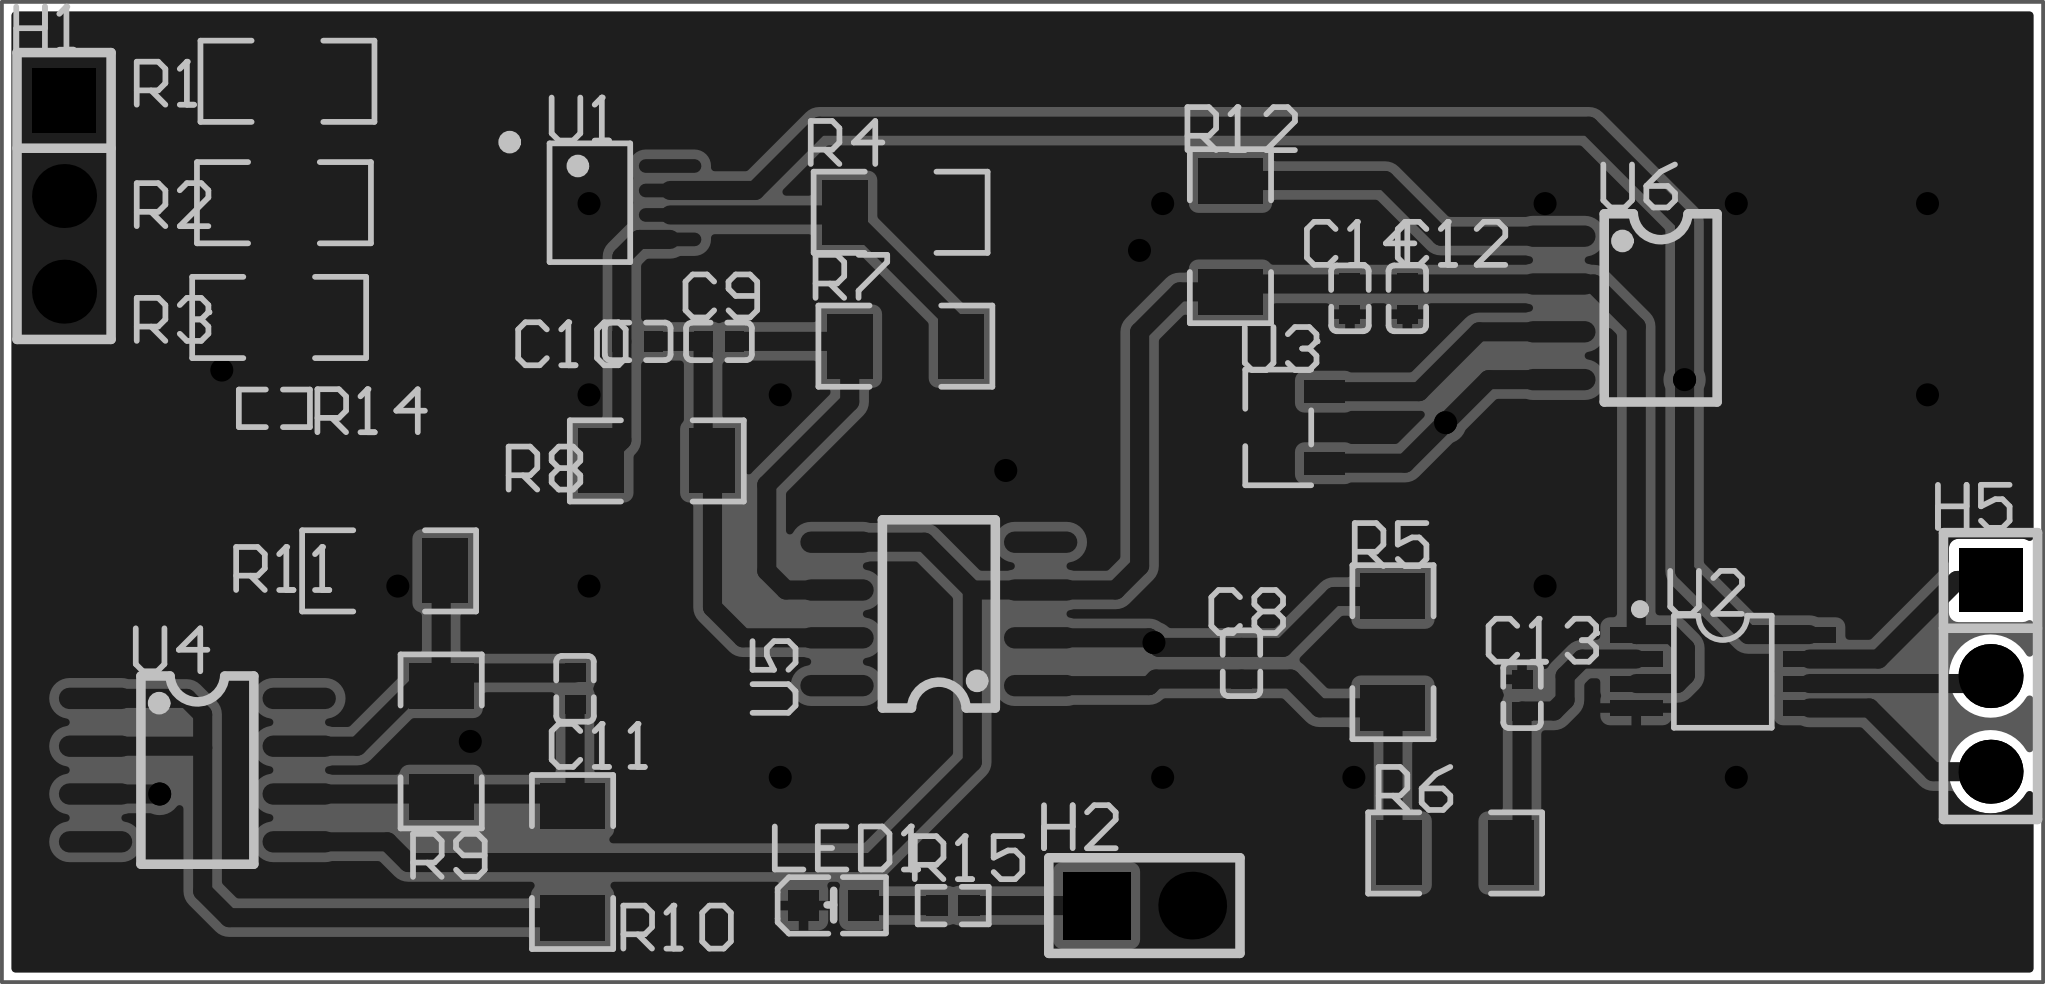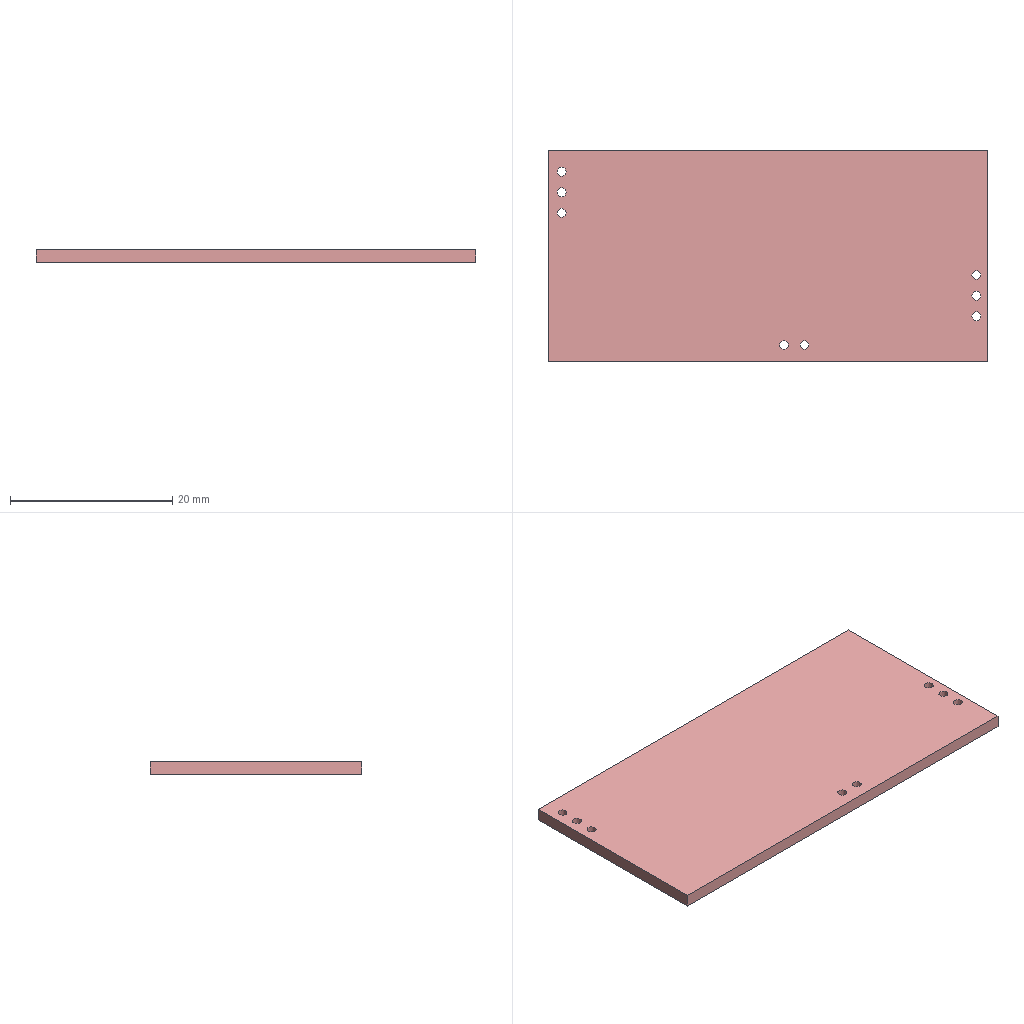Circuit board layout | Altium Designer | box 54.2 x 26 x 1.6 mm
Layer stack:
# Altium Designer layer stack of  (unit mm; dielectric type: 0 none, 1 core, 2 prepreg, 3 surface material)
index,name,kind,layer,copper_thickness_mm,dielectric_type,dielectric_thickness_mm,dielectric_material,dielectric_constant
0,Top Paste Mask Layer,other,,,,,,
1,Top Silkscreen Layer,other,,,,,,
2,Top Solder Mask Layer,dielectric,,,3,0.01,,3.3
3,Top Layer,copper,Top Layer,0.035,,,,
4,Dielectric1,dielectric,,,3,1.51,FR4,4.5
5,Bottom Layer,copper,Bottom Layer,0.035,,,,
6,Bottom Solder Mask Layer,dielectric,,,3,0.01,,3.3
7,Bottom Silkscreen Layer,other,,,,,,
8,Bottom Paste Mask Layer,other,,,,,,
# drill layer pairs: low layer,high layer
drill_pair,Top Layer,Bottom Layer
Part placement:
Designator,Comment,Layer,Footprint,Center-X(mm),Center-Y(mm),Rotation
C8,0.0015uF,TopLayer,C0402,112.307,89.242,270
C9,1uF,TopLayer,C0402,98.425,97.79,0
C10,750pF,TopLayer,C0402,96.266,97.79,0
C11,39pF,TopLayer,C0402,94.601,88.562,270
C12,0.1uF,TopLayer,C0402,116.713,98.933,90
C13,0.1uF,TopLayer,C0402,119.761,88.392,270
C14,10uF,TopLayer,C0402,115.189,98.933,270
H1,,TopLayer,HDR-TH_3P-P2.54-V-M,81.026,101.65,270
H2,,TopLayer,HDR-TH_2P-P2.54-V-M-1,109.728,82.804,0
H5,,TopLayer,HDR-TH_3P-P2.54-V-M,132.207,88.9,270
LED1,KT-0603W,TopLayer,LED0603-R-RD_WHITE,101.473,82.804,0
R1,390kΩ,TopLayer,R1206,86.961,104.698,0
R2,40kΩ,TopLayer,R1206,86.868,101.473,0
R3,40kΩ,TopLayer,R1206,86.741,98.425,0
R4,5kΩ,TopLayer,R1206,103.251,101.219,0
R5,1MΩ,TopLayer,R1206,116.332,89.535,270
R6,100Ω,TopLayer,R1206,117.983,84.201,0
R7,3.2MΩ,TopLayer,R1206,103.378,97.663,0
R8,200kΩ,TopLayer,R1206,96.774,94.615,0
R9,390kΩ,TopLayer,R1206,91.045,87.165,270
R10,20kΩ,TopLayer,R1206,94.536,83.961,270
R11,390kΩ,TopLayer,R1206,89.662,91.694,0
R12,100Ω,TopLayer,R1206,112.014,100.584,270
R14,390kΩ,TopLayer,R0402,86.614,96.012,0
R15,1.15kΩ,TopLayer,R0402,104.648,82.804,0
U1,INA326EA/2K5,TopLayer,VSSOP-8_L3.0-W3.0-P0.65-LS5.0-BL,94.996,101.473,270
U2,ADS8321E/2K5,TopLayer,MSOP-8_L3.0-W3.0-P0.65-LS4.9-BL,125.095,89.027,270
U3,REF3125AIDBZR,TopLayer,SOT-23-3_L2.9-W1.6-P1.90-LS2.8-BR,113.284,95.504,0
U4,OPA2335AIDR,TopLayer,SOIC-8_L5.0-W4.0-P1.27-LS6.0-BL,84.568,86.403,270
U5,OPA2335AIDR,TopLayer,SOIC-8_L5.0-W4.0-P1.27-LS6.0-BL,104.267,90.551,90
U6,OPA2335AIDR,TopLayer,SOIC-8_L5.0-W4.0-P1.27-LS6.0-BL,123.444,98.679,270
Pad and via stacks:
# Altium Designer via and pad stacks of  (unit mm). Each distinct definition once, with the count of objects using it.
# via: kind,start_layer,end_layer,hole_mm,diameter_mm,mode(0 simple;1 top-mid-bottom;2 full stack),diameter_per_layer,count,example_net
# pad: kind,layer,hole_mm,hole_type(0 round;1 square;2 slot),plating,top_size,top_shape(1 round;2 rect;3 octagon;9 rounded rect),mid_size,bottom_size,mode,footprint,size_per_layer,count,example
pad,Top Layer,0,0,plated,0.5x0.54,2,0.5x0.54,0.5x0.54,0,C0402,,14,C8.2
pad,Top Layer,0,0,plated,0.8x0.8,2,0.8x0.8,0.8x0.8,0,LED0603-R-RD_WHITE,,2,LED1.2
pad,Top Layer,0,0,plated,1.208x1.701,2,1.208x1.701,1.208x1.701,0,R1206,,24,R1.2
pad,Top Layer,0,0,plated,0.5657x0.54,2,0.5657x0.54,0.5657x0.54,0,R0402,,4,R14.2
pad,Top Layer,0,0,plated,0.364x1.662,1,0.364x1.662,0.364x1.662,0,VSSOP-8_L3.0-W3.0-P0.65-LS5.0-BL,,8,U1.1
pad,Top Layer,0,0,plated,0.406x1.397,2,0.406x1.397,0.406x1.397,0,MSOP-8_L3.0-W3.0-P0.65-LS4.9-BL,,8,U2.1
pad,Top Layer,0,0,plated,1.07x0.6,2,1.07x0.6,1.07x0.6,0,SOT-23-3_L2.9-W1.6-P1.90-LS2.8-BR,,3,U3.1
pad,Top Layer,0,0,plated,0.5684x1.95,1,0.5684x1.95,0.5684x1.95,0,SOIC-8_L5.0-W4.0-P1.27-LS6.0-BL,,24,U4.1
pad,Multi-Layer,1.1,0,plated,1.7x1.7,2,1.7x1.7,1.7x1.7,0,HDR-TH_3P-P2.54-V-M,,2,H1.1
pad,Multi-Layer,1.1,0,plated,1.7x1.7,1,1.7x1.7,1.7x1.7,0,HDR-TH_3P-P2.54-V-M,,4,H1.2
pad,Multi-Layer,1.1,0,plated,1.8x1.8,1,1.8x1.8,1.8x1.8,0,HDR-TH_2P-P2.54-V-M-1,,1,H2.2
pad,Multi-Layer,1.1,0,plated,1.8x1.8,2,1.8x1.8,1.8x1.8,0,HDR-TH_2P-P2.54-V-M-1,,1,H2.1
via,Top Layer,Bottom Layer,0.3048,0.61,0,,23,$1N41
Copper pours:
name,layer,net,type(0 solid;1 hatched;2 none)
Top Layer-GND,Top Layer,GND,0
Bottom Layer-GND,Bottom Layer,GND,0